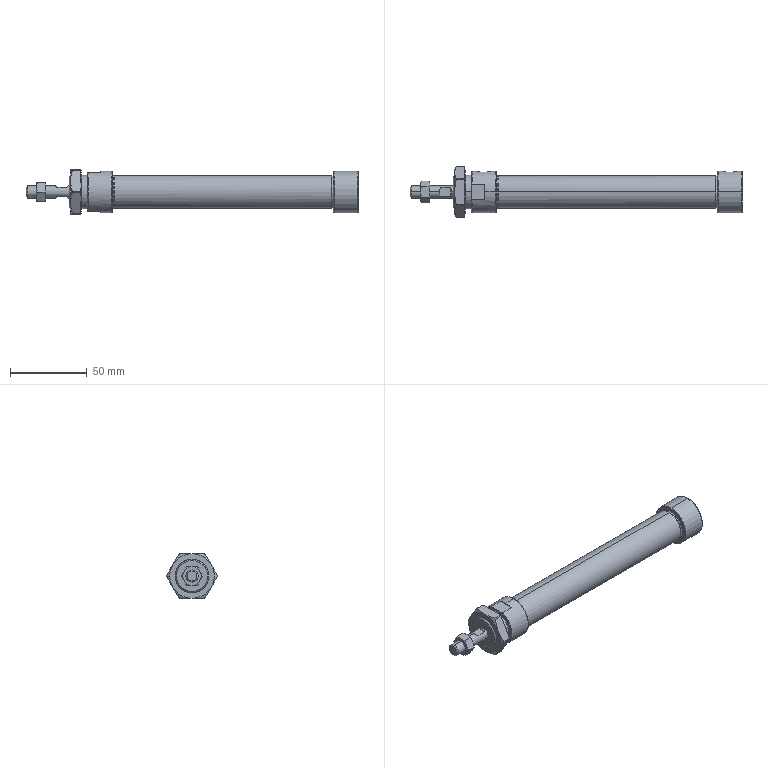Part | SolidWorks | features BaseBody 4, MoveFace 2 | 4 solids | 125 faces | box 216 x 33 x 29 mm | volume 70074 mm3 | plane 41 | cone 40 | cylinder 36 | spline 8 | commonest cylinder face diameters 21.4 x6 33 x6 8 x4 8.566 x4 27 x4 6.647 x2